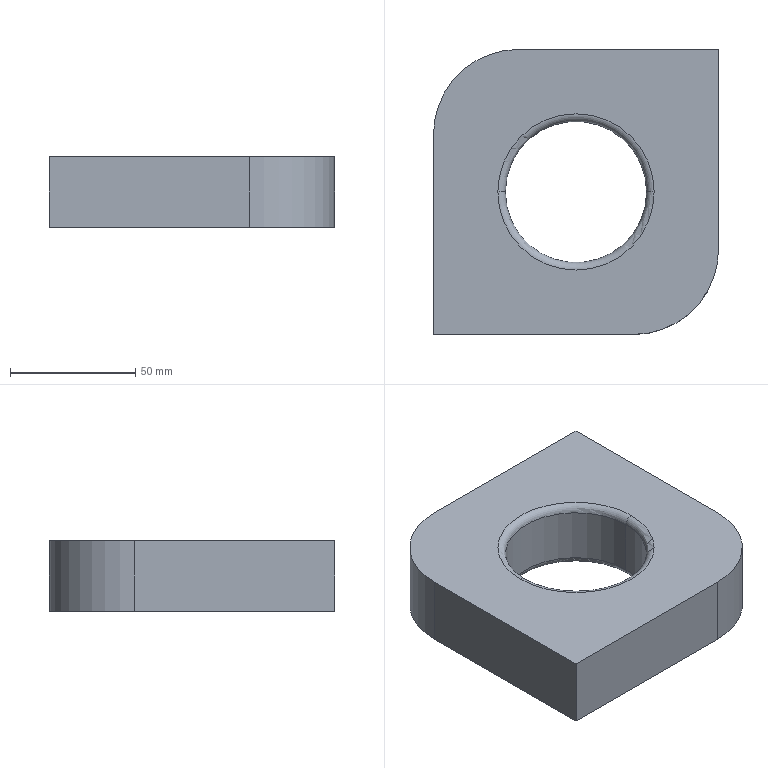Part | SolidWorks | features Fillet 2, Extrusion 1 | 1 solid | 14 faces | box 114 x 114 x 28 mm | volume 279092 mm3 | plane 6 | torus 4 | cylinder 4 | commonest cylinder face diameters 56.5 x2 68 x2
STEP:
#1=CARTESIAN_POINT('',(-31.25,0.,28.));
#2=VERTEX_POINT('',#1);
#3=CARTESIAN_POINT('',(31.25,0.,28.));
#4=VERTEX_POINT('',#3);
#5=CARTESIAN_POINT('',(0.,0.,28.));
#6=DIRECTION('',(0.,0.,-1.));
#7=DIRECTION('',(1.,0.,0.));
#8=AXIS2_PLACEMENT_3D('',#5,#6,#7);
#9=CIRCLE('',#8,31.25);
#10=EDGE_CURVE('',#2,#4,#9,.T.);
#11=ORIENTED_EDGE('',*,*,#10,.F.);
#12=CARTESIAN_POINT('',(-28.25,0.,25.));
#13=VERTEX_POINT('',#12);
#14=CARTESIAN_POINT('',(-31.25,0.,25.));
#15=DIRECTION('',(0.,1.,0.));
#16=DIRECTION('',(-1.,0.,0.));
#17=AXIS2_PLACEMENT_3D('',#14,#15,#16);
#18=CIRCLE('',#17,3.);
#19=EDGE_CURVE('',#2,#13,#18,.T.);
#20=ORIENTED_EDGE('',*,*,#19,.T.);
#21=CARTESIAN_POINT('',(28.25,0.,25.));
#22=VERTEX_POINT('',#21);
#23=CARTESIAN_POINT('',(0.,0.,25.));
#24=DIRECTION('',(0.,0.,1.));
#25=DIRECTION('',(1.,0.,0.));
#26=AXIS2_PLACEMENT_3D('',#23,#24,#25);
#27=CIRCLE('',#26,28.25);
#28=EDGE_CURVE('',#22,#13,#27,.T.);
#29=ORIENTED_EDGE('',*,*,#28,.F.);
#30=CARTESIAN_POINT('',(31.25,0.,25.));
#31=DIRECTION('',(0.,-1.,0.));
#32=DIRECTION('',(0.,0.,-1.));
#33=AXIS2_PLACEMENT_3D('',#30,#31,#32);
#34=CIRCLE('',#33,3.);
#35=EDGE_CURVE('',#4,#22,#34,.T.);
#36=ORIENTED_EDGE('',*,*,#35,.F.);
#37=EDGE_LOOP('',(#11,#20,#29,#36));
#38=FACE_OUTER_BOUND('',#37,.T.);
#39=CARTESIAN_POINT('',(0.,0.,25.));
#40=DIRECTION('',(0.,0.,1.));
#41=DIRECTION('',(1.,0.,0.));
#42=AXIS2_PLACEMENT_3D('',#39,#40,#41);
#43=TOROIDAL_SURFACE('',#42,31.25,3.);
#44=ADVANCED_FACE('',(#38),#43,.T.);
#45=CARTESIAN_POINT('',(-28.25,0.,3.));
#46=VERTEX_POINT('',#45);
#47=CARTESIAN_POINT('',(28.25,0.,3.));
#48=VERTEX_POINT('',#47);
#49=CARTESIAN_POINT('',(0.,0.,3.));
#50=DIRECTION('',(0.,0.,-1.));
#51=DIRECTION('',(1.,0.,0.));
#52=AXIS2_PLACEMENT_3D('',#49,#50,#51);
#53=CIRCLE('',#52,28.25);
#54=EDGE_CURVE('',#46,#48,#53,.T.);
#55=ORIENTED_EDGE('',*,*,#54,.F.);
#56=CARTESIAN_POINT('',(-31.25,0.,0.));
#57=VERTEX_POINT('',#56);
#58=CARTESIAN_POINT('',(-31.25,0.,3.));
#59=DIRECTION('',(0.,1.,0.));
#60=DIRECTION('',(-1.,0.,0.));
#61=AXIS2_PLACEMENT_3D('',#58,#59,#60);
#62=CIRCLE('',#61,3.);
#63=EDGE_CURVE('',#46,#57,#62,.T.);
#64=ORIENTED_EDGE('',*,*,#63,.T.);
#65=CARTESIAN_POINT('',(31.25,0.,0.));
#66=VERTEX_POINT('',#65);
#67=CARTESIAN_POINT('',(0.,0.,0.));
#68=DIRECTION('',(0.,0.,1.));
#69=DIRECTION('',(1.,0.,0.));
#70=AXIS2_PLACEMENT_3D('',#67,#68,#69);
#71=CIRCLE('',#70,31.25);
#72=EDGE_CURVE('',#66,#57,#71,.T.);
#73=ORIENTED_EDGE('',*,*,#72,.F.);
#74=CARTESIAN_POINT('',(31.25,0.,3.));
#75=DIRECTION('',(0.,-1.,0.));
#76=DIRECTION('',(0.,0.,-1.));
#77=AXIS2_PLACEMENT_3D('',#74,#75,#76);
#78=CIRCLE('',#77,3.);
#79=EDGE_CURVE('',#48,#66,#78,.T.);
#80=ORIENTED_EDGE('',*,*,#79,.F.);
#81=EDGE_LOOP('',(#55,#64,#73,#80));
#82=FACE_OUTER_BOUND('',#81,.T.);
#83=CARTESIAN_POINT('',(0.,0.,3.));
#84=DIRECTION('',(0.,0.,1.));
#85=DIRECTION('',(1.,0.,0.));
#86=AXIS2_PLACEMENT_3D('',#83,#84,#85);
#87=TOROIDAL_SURFACE('',#86,31.25,3.);
#88=ADVANCED_FACE('',(#82),#87,.T.);
#89=CARTESIAN_POINT('',(0.,0.,25.));
#90=DIRECTION('',(0.,0.,1.));
#91=DIRECTION('',(1.,0.,0.));
#92=AXIS2_PLACEMENT_3D('',#89,#90,#91);
#93=CIRCLE('',#92,28.25);
#94=EDGE_CURVE('',#13,#22,#93,.T.);
#95=ORIENTED_EDGE('',*,*,#94,.T.);
#96=CARTESIAN_POINT('',(28.25,0.,28.));
#97=DIRECTION('',(0.,0.,-1.));
#98=VECTOR('',#97,1000.);
#99=LINE('',#96,#98);
#100=EDGE_CURVE('',#22,#48,#99,.T.);
#101=ORIENTED_EDGE('',*,*,#100,.T.);
#102=CARTESIAN_POINT('',(0.,0.,3.));
#103=DIRECTION('',(0.,0.,-1.));
#104=DIRECTION('',(1.,0.,0.));
#105=AXIS2_PLACEMENT_3D('',#102,#103,#104);
#106=CIRCLE('',#105,28.25);
#107=EDGE_CURVE('',#48,#46,#106,.T.);
#108=ORIENTED_EDGE('',*,*,#107,.T.);
#109=CARTESIAN_POINT('',(-28.25,0.,28.));
#110=DIRECTION('',(0.,0.,-1.));
#111=VECTOR('',#110,1000.);
#112=LINE('',#109,#111);
#113=EDGE_CURVE('',#13,#46,#112,.T.);
#114=ORIENTED_EDGE('',*,*,#113,.F.);
#115=EDGE_LOOP('',(#95,#101,#108,#114));
#116=FACE_OUTER_BOUND('',#115,.T.);
#117=CARTESIAN_POINT('',(0.,0.,28.));
#118=DIRECTION('',(0.,0.,-1.));
#119=DIRECTION('',(-1.,0.,0.));
#120=AXIS2_PLACEMENT_3D('',#117,#118,#119);
#121=CYLINDRICAL_SURFACE('',#120,28.25);
#122=ADVANCED_FACE('',(#116),#121,.F.);
#123=CARTESIAN_POINT('',(0.,0.,28.));
#124=DIRECTION('',(0.,0.,-1.));
#125=DIRECTION('',(1.,0.,0.));
#126=AXIS2_PLACEMENT_3D('',#123,#124,#125);
#127=CIRCLE('',#126,31.25);
#128=EDGE_CURVE('',#4,#2,#127,.T.);
#129=ORIENTED_EDGE('',*,*,#128,.T.);
#130=ORIENTED_EDGE('',*,*,#10,.T.);
#131=EDGE_LOOP('',(#129,#130));
#132=FACE_BOUND('',#131,.T.);
#133=CARTESIAN_POINT('',(-57.,-57.,28.));
#134=VERTEX_POINT('',#133);
#135=CARTESIAN_POINT('',(23.,-57.,28.));
#136=VERTEX_POINT('',#135);
#137=CARTESIAN_POINT('',(-57.,-57.,28.));
#138=DIRECTION('',(1.,0.,0.));
#139=VECTOR('',#138,1000.);
#140=LINE('',#137,#139);
#141=EDGE_CURVE('',#134,#136,#140,.T.);
#142=ORIENTED_EDGE('',*,*,#141,.T.);
#143=CARTESIAN_POINT('',(57.,-23.,28.));
#144=VERTEX_POINT('',#143);
#145=CARTESIAN_POINT('',(23.,-23.,28.));
#146=DIRECTION('',(0.,0.,1.));
#147=DIRECTION('',(1.,0.,0.));
#148=AXIS2_PLACEMENT_3D('',#145,#146,#147);
#149=CIRCLE('',#148,34.);
#150=EDGE_CURVE('',#136,#144,#149,.T.);
#151=ORIENTED_EDGE('',*,*,#150,.T.);
#152=CARTESIAN_POINT('',(57.,57.,28.));
#153=VERTEX_POINT('',#152);
#154=CARTESIAN_POINT('',(57.,57.,28.));
#155=DIRECTION('',(0.,1.,0.));
#156=VECTOR('',#155,1000.);
#157=LINE('',#154,#156);
#158=EDGE_CURVE('',#144,#153,#157,.T.);
#159=ORIENTED_EDGE('',*,*,#158,.T.);
#160=CARTESIAN_POINT('',(-23.,57.,28.));
#161=VERTEX_POINT('',#160);
#162=CARTESIAN_POINT('',(-57.,57.,28.));
#163=DIRECTION('',(-1.,0.,0.));
#164=VECTOR('',#163,1000.);
#165=LINE('',#162,#164);
#166=EDGE_CURVE('',#153,#161,#165,.T.);
#167=ORIENTED_EDGE('',*,*,#166,.T.);
#168=CARTESIAN_POINT('',(-57.,23.,28.));
#169=VERTEX_POINT('',#168);
#170=CARTESIAN_POINT('',(-23.,23.,28.));
#171=DIRECTION('',(0.,0.,1.));
#172=DIRECTION('',(1.,0.,0.));
#173=AXIS2_PLACEMENT_3D('',#170,#171,#172);
#174=CIRCLE('',#173,34.);
#175=EDGE_CURVE('',#161,#169,#174,.T.);
#176=ORIENTED_EDGE('',*,*,#175,.T.);
#177=CARTESIAN_POINT('',(-57.,57.,28.));
#178=DIRECTION('',(0.,-1.,0.));
#179=VECTOR('',#178,1000.);
#180=LINE('',#177,#179);
#181=EDGE_CURVE('',#169,#134,#180,.T.);
#182=ORIENTED_EDGE('',*,*,#181,.T.);
#183=EDGE_LOOP('',(#142,#151,#159,#167,#176,#182));
#184=FACE_OUTER_BOUND('',#183,.T.);
#185=CARTESIAN_POINT('',(0.,0.,28.));
#186=DIRECTION('',(0.,0.,1.));
#187=DIRECTION('',(1.,0.,0.));
#188=AXIS2_PLACEMENT_3D('',#185,#186,#187);
#189=PLANE('',#188);
#190=ADVANCED_FACE('',(#132,#184),#189,.T.);
#191=ORIENTED_EDGE('',*,*,#72,.T.);
#192=CARTESIAN_POINT('',(0.,0.,0.));
#193=DIRECTION('',(0.,0.,1.));
#194=DIRECTION('',(1.,0.,0.));
#195=AXIS2_PLACEMENT_3D('',#192,#193,#194);
#196=CIRCLE('',#195,31.25);
#197=EDGE_CURVE('',#57,#66,#196,.T.);
#198=ORIENTED_EDGE('',*,*,#197,.T.);
#199=EDGE_LOOP('',(#191,#198));
#200=FACE_BOUND('',#199,.T.);
#201=CARTESIAN_POINT('',(57.,-23.,0.));
#202=VERTEX_POINT('',#201);
#203=CARTESIAN_POINT('',(57.,57.,0.));
#204=VERTEX_POINT('',#203);
#205=CARTESIAN_POINT('',(57.,57.,0.));
#206=DIRECTION('',(0.,1.,0.));
#207=VECTOR('',#206,1000.);
#208=LINE('',#205,#207);
#209=EDGE_CURVE('',#202,#204,#208,.T.);
#210=ORIENTED_EDGE('',*,*,#209,.F.);
#211=CARTESIAN_POINT('',(23.,-57.,0.));
#212=VERTEX_POINT('',#211);
#213=CARTESIAN_POINT('',(23.,-23.,0.));
#214=DIRECTION('',(0.,0.,-1.));
#215=DIRECTION('',(1.,0.,0.));
#216=AXIS2_PLACEMENT_3D('',#213,#214,#215);
#217=CIRCLE('',#216,34.);
#218=EDGE_CURVE('',#202,#212,#217,.T.);
#219=ORIENTED_EDGE('',*,*,#218,.T.);
#220=CARTESIAN_POINT('',(-57.,-57.,0.));
#221=VERTEX_POINT('',#220);
#222=CARTESIAN_POINT('',(-57.,-57.,0.));
#223=DIRECTION('',(1.,0.,0.));
#224=VECTOR('',#223,1000.);
#225=LINE('',#222,#224);
#226=EDGE_CURVE('',#221,#212,#225,.T.);
#227=ORIENTED_EDGE('',*,*,#226,.F.);
#228=CARTESIAN_POINT('',(-57.,23.,0.));
#229=VERTEX_POINT('',#228);
#230=CARTESIAN_POINT('',(-57.,57.,0.));
#231=DIRECTION('',(0.,-1.,0.));
#232=VECTOR('',#231,1000.);
#233=LINE('',#230,#232);
#234=EDGE_CURVE('',#229,#221,#233,.T.);
#235=ORIENTED_EDGE('',*,*,#234,.F.);
#236=CARTESIAN_POINT('',(-23.,57.,0.));
#237=VERTEX_POINT('',#236);
#238=CARTESIAN_POINT('',(-23.,23.,0.));
#239=DIRECTION('',(0.,0.,-1.));
#240=DIRECTION('',(1.,0.,0.));
#241=AXIS2_PLACEMENT_3D('',#238,#239,#240);
#242=CIRCLE('',#241,34.);
#243=EDGE_CURVE('',#229,#237,#242,.T.);
#244=ORIENTED_EDGE('',*,*,#243,.T.);
#245=CARTESIAN_POINT('',(-57.,57.,0.));
#246=DIRECTION('',(-1.,0.,0.));
#247=VECTOR('',#246,1000.);
#248=LINE('',#245,#247);
#249=EDGE_CURVE('',#204,#237,#248,.T.);
#250=ORIENTED_EDGE('',*,*,#249,.F.);
#251=EDGE_LOOP('',(#210,#219,#227,#235,#244,#250));
#252=FACE_OUTER_BOUND('',#251,.T.);
#253=CARTESIAN_POINT('',(0.,0.,0.));
#254=DIRECTION('',(0.,0.,1.));
#255=DIRECTION('',(1.,0.,0.));
#256=AXIS2_PLACEMENT_3D('',#253,#254,#255);
#257=PLANE('',#256);
#258=ADVANCED_FACE('',(#200,#252),#257,.F.);
#259=ORIENTED_EDGE('',*,*,#181,.F.);
#260=CARTESIAN_POINT('',(-57.,23.,28.));
#261=DIRECTION('',(0.,0.,-1.));
#262=VECTOR('',#261,1000.);
#263=LINE('',#260,#262);
#264=EDGE_CURVE('',#169,#229,#263,.T.);
#265=ORIENTED_EDGE('',*,*,#264,.T.);
#266=ORIENTED_EDGE('',*,*,#234,.T.);
#267=CARTESIAN_POINT('',(-57.,-57.,28.));
#268=DIRECTION('',(0.,0.,-1.));
#269=VECTOR('',#268,1000.);
#270=LINE('',#267,#269);
#271=EDGE_CURVE('',#134,#221,#270,.T.);
#272=ORIENTED_EDGE('',*,*,#271,.F.);
#273=EDGE_LOOP('',(#259,#265,#266,#272));
#274=FACE_OUTER_BOUND('',#273,.T.);
#275=CARTESIAN_POINT('',(-57.,57.,28.));
#276=DIRECTION('',(1.,0.,0.));
#277=DIRECTION('',(0.,1.,0.));
#278=AXIS2_PLACEMENT_3D('',#275,#276,#277);
#279=PLANE('',#278);
#280=ADVANCED_FACE('',(#274),#279,.F.);
#281=ORIENTED_EDGE('',*,*,#226,.T.);
#282=CARTESIAN_POINT('',(23.,-57.,28.));
#283=DIRECTION('',(0.,0.,1.));
#284=VECTOR('',#283,1000.);
#285=LINE('',#282,#284);
#286=EDGE_CURVE('',#212,#136,#285,.T.);
#287=ORIENTED_EDGE('',*,*,#286,.T.);
#288=ORIENTED_EDGE('',*,*,#141,.F.);
#289=ORIENTED_EDGE('',*,*,#271,.T.);
#290=EDGE_LOOP('',(#281,#287,#288,#289));
#291=FACE_OUTER_BOUND('',#290,.T.);
#292=CARTESIAN_POINT('',(-57.,-57.,28.));
#293=DIRECTION('',(0.,1.,0.));
#294=DIRECTION('',(0.,0.,1.));
#295=AXIS2_PLACEMENT_3D('',#292,#293,#294);
#296=PLANE('',#295);
#297=ADVANCED_FACE('',(#291),#296,.F.);
#298=ORIENTED_EDGE('',*,*,#158,.F.);
#299=CARTESIAN_POINT('',(57.,-23.,28.));
#300=DIRECTION('',(0.,0.,-1.));
#301=VECTOR('',#300,1000.);
#302=LINE('',#299,#301);
#303=EDGE_CURVE('',#144,#202,#302,.T.);
#304=ORIENTED_EDGE('',*,*,#303,.T.);
#305=ORIENTED_EDGE('',*,*,#209,.T.);
#306=CARTESIAN_POINT('',(57.,57.,28.));
#307=DIRECTION('',(0.,0.,-1.));
#308=VECTOR('',#307,1000.);
#309=LINE('',#306,#308);
#310=EDGE_CURVE('',#153,#204,#309,.T.);
#311=ORIENTED_EDGE('',*,*,#310,.F.);
#312=EDGE_LOOP('',(#298,#304,#305,#311));
#313=FACE_OUTER_BOUND('',#312,.T.);
#314=CARTESIAN_POINT('',(57.,57.,28.));
#315=DIRECTION('',(-1.,0.,0.));
#316=DIRECTION('',(0.,-1.,0.));
#317=AXIS2_PLACEMENT_3D('',#314,#315,#316);
#318=PLANE('',#317);
#319=ADVANCED_FACE('',(#313),#318,.F.);
#320=ORIENTED_EDGE('',*,*,#249,.T.);
#321=CARTESIAN_POINT('',(-23.,57.,28.));
#322=DIRECTION('',(0.,0.,1.));
#323=VECTOR('',#322,1000.);
#324=LINE('',#321,#323);
#325=EDGE_CURVE('',#237,#161,#324,.T.);
#326=ORIENTED_EDGE('',*,*,#325,.T.);
#327=ORIENTED_EDGE('',*,*,#166,.F.);
#328=ORIENTED_EDGE('',*,*,#310,.T.);
#329=EDGE_LOOP('',(#320,#326,#327,#328));
#330=FACE_OUTER_BOUND('',#329,.T.);
#331=CARTESIAN_POINT('',(-57.,57.,28.));
#332=DIRECTION('',(0.,-1.,0.));
#333=DIRECTION('',(0.,0.,-1.));
#334=AXIS2_PLACEMENT_3D('',#331,#332,#333);
#335=PLANE('',#334);
#336=ADVANCED_FACE('',(#330),#335,.F.);
#337=ORIENTED_EDGE('',*,*,#100,.F.);
#338=ORIENTED_EDGE('',*,*,#28,.T.);
#339=ORIENTED_EDGE('',*,*,#113,.T.);
#340=ORIENTED_EDGE('',*,*,#54,.T.);
#341=EDGE_LOOP('',(#337,#338,#339,#340));
#342=FACE_OUTER_BOUND('',#341,.T.);
#343=CARTESIAN_POINT('',(0.,0.,28.));
#344=DIRECTION('',(0.,0.,-1.));
#345=DIRECTION('',(-1.,0.,0.));
#346=AXIS2_PLACEMENT_3D('',#343,#344,#345);
#347=CYLINDRICAL_SURFACE('',#346,28.25);
#348=ADVANCED_FACE('',(#342),#347,.F.);
#349=ORIENTED_EDGE('',*,*,#63,.F.);
#350=ORIENTED_EDGE('',*,*,#107,.F.);
#351=ORIENTED_EDGE('',*,*,#79,.T.);
#352=ORIENTED_EDGE('',*,*,#197,.F.);
#353=EDGE_LOOP('',(#349,#350,#351,#352));
#354=FACE_OUTER_BOUND('',#353,.T.);
#355=CARTESIAN_POINT('',(0.,0.,3.));
#356=DIRECTION('',(0.,0.,1.));
#357=DIRECTION('',(1.,0.,0.));
#358=AXIS2_PLACEMENT_3D('',#355,#356,#357);
#359=TOROIDAL_SURFACE('',#358,31.25,3.);
#360=ADVANCED_FACE('',(#354),#359,.T.);
#361=ORIENTED_EDGE('',*,*,#19,.F.);
#362=ORIENTED_EDGE('',*,*,#128,.F.);
#363=ORIENTED_EDGE('',*,*,#35,.T.);
#364=ORIENTED_EDGE('',*,*,#94,.F.);
#365=EDGE_LOOP('',(#361,#362,#363,#364));
#366=FACE_OUTER_BOUND('',#365,.T.);
#367=CARTESIAN_POINT('',(0.,0.,25.));
#368=DIRECTION('',(0.,0.,1.));
#369=DIRECTION('',(1.,0.,0.));
#370=AXIS2_PLACEMENT_3D('',#367,#368,#369);
#371=TOROIDAL_SURFACE('',#370,31.25,3.);
#372=ADVANCED_FACE('',(#366),#371,.T.);
#373=ORIENTED_EDGE('',*,*,#150,.F.);
#374=ORIENTED_EDGE('',*,*,#286,.F.);
#375=ORIENTED_EDGE('',*,*,#218,.F.);
#376=ORIENTED_EDGE('',*,*,#303,.F.);
#377=EDGE_LOOP('',(#373,#374,#375,#376));
#378=FACE_OUTER_BOUND('',#377,.T.);
#379=CARTESIAN_POINT('',(23.,-23.,28.));
#380=DIRECTION('',(0.,0.,-1.));
#381=DIRECTION('',(-1.,0.,0.));
#382=AXIS2_PLACEMENT_3D('',#379,#380,#381);
#383=CYLINDRICAL_SURFACE('',#382,34.);
#384=ADVANCED_FACE('',(#378),#383,.T.);
#385=ORIENTED_EDGE('',*,*,#175,.F.);
#386=ORIENTED_EDGE('',*,*,#325,.F.);
#387=ORIENTED_EDGE('',*,*,#243,.F.);
#388=ORIENTED_EDGE('',*,*,#264,.F.);
#389=EDGE_LOOP('',(#385,#386,#387,#388));
#390=FACE_OUTER_BOUND('',#389,.T.);
#391=CARTESIAN_POINT('',(-23.,23.,28.));
#392=DIRECTION('',(0.,0.,-1.));
#393=DIRECTION('',(-1.,0.,0.));
#394=AXIS2_PLACEMENT_3D('',#391,#392,#393);
#395=CYLINDRICAL_SURFACE('',#394,34.);
#396=ADVANCED_FACE('',(#390),#395,.T.);
#397=CLOSED_SHELL('',(#44,#88,#122,#190,#258,#280,#297,#319,#336,#348,#360,#372,#384,#396));
#398=MANIFOLD_SOLID_BREP('',#397);
#399=CARTESIAN_POINT('',(0.,0.,0.));
#400=DIRECTION('',(0.,0.,1.));
#401=DIRECTION('',(1.,0.,0.));
#402=AXIS2_PLACEMENT_3D('',#399,#400,#401);
#403=(LENGTH_UNIT()NAMED_UNIT(*)SI_UNIT(.MILLI.,.METRE.));
#404=UNCERTAINTY_MEASURE_WITH_UNIT(LENGTH_MEASURE(0.00001),#403,'','');
#405=(NAMED_UNIT(*)PLANE_ANGLE_UNIT()SI_UNIT($,.RADIAN.));
#406=(NAMED_UNIT(*)SI_UNIT($,.STERADIAN.)SOLID_ANGLE_UNIT());
#407=(GEOMETRIC_REPRESENTATION_CONTEXT(3)GLOBAL_UNCERTAINTY_ASSIGNED_CONTEXT((#404))GLOBAL_UNIT_ASSIGNED_CONTEXT((#403,#405,#406))REPRESENTATION_CONTEXT('',''));
#408=ADVANCED_BREP_SHAPE_REPRESENTATION('',(#398,#402),#407);